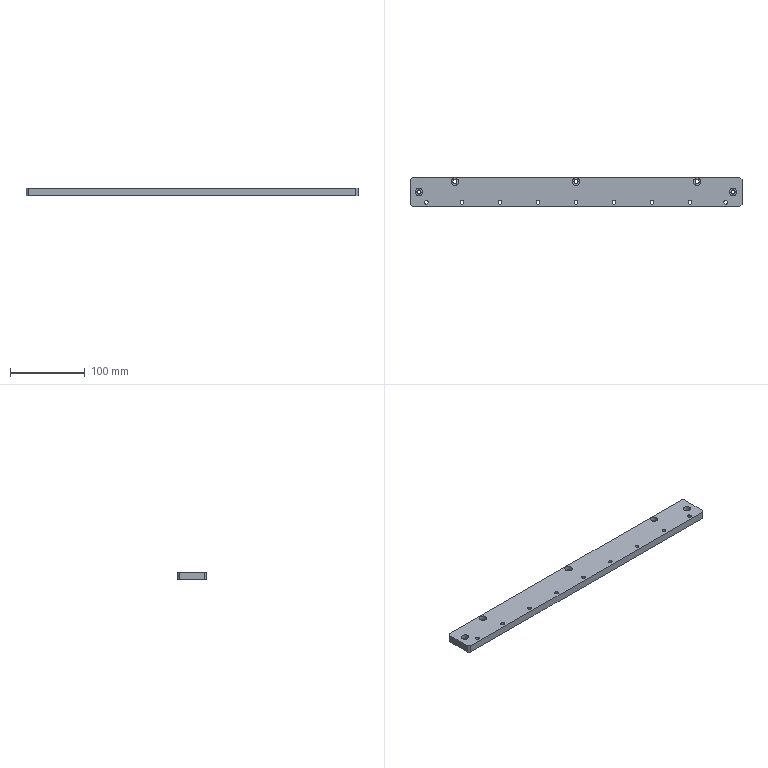Part | STEP file | PN_0021 | 1 solid | 53 faces | box 444 x 40 x 10 mm | volume 172920 mm3 | cylinder 38 | plane 15 | commonest cylinder face diameters 5 x18 5.5 x10 10 x10